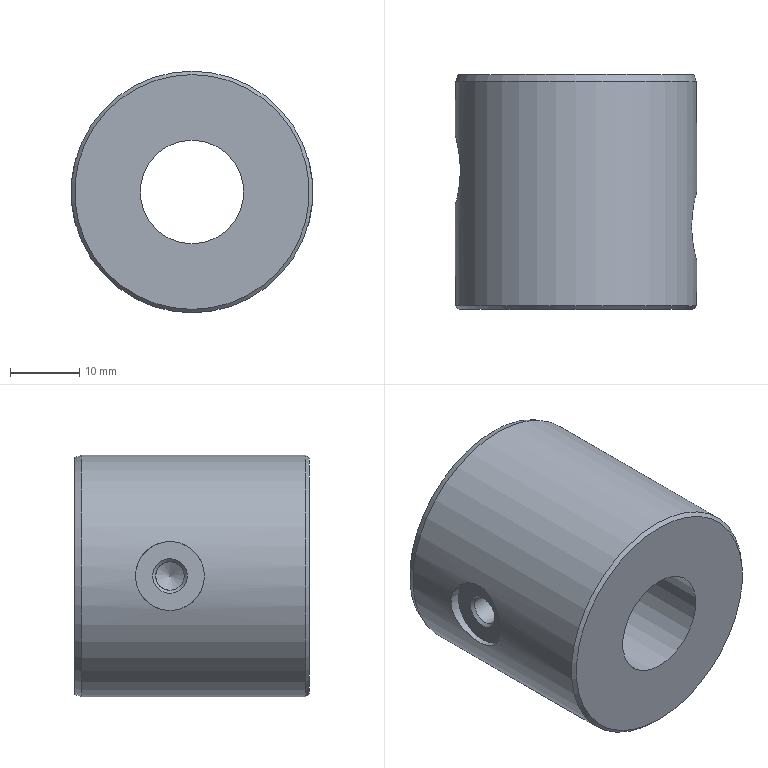Part | NX | 1 solid | 22 faces | box 35 x 34 x 35 mm | volume 26297 mm3 | cone 10 | cylinder 8 | plane 4 | commonest cylinder face diameters 2.459 x2 4.134 x2 10 x2 15 x1 35 x1
STEP:
#1=CARTESIAN_POINT('',(0.,14.5,-17.5));
#2=VERTEX_POINT('',#1);
#3=CARTESIAN_POINT('',(0.,14.5,0.));
#4=DIRECTION('',(0.,-1.,0.));
#5=DIRECTION('',(0.,0.,-1.));
#6=AXIS2_PLACEMENT_3D('',#3,#4,#5);
#7=CIRCLE('',#6,17.5);
#8=EDGE_CURVE('',#2,#2,#7,.F.);
#9=ORIENTED_EDGE('',*,*,#8,.T.);
#10=EDGE_LOOP('',(#9));
#11=FACE_BOUND('',#10,.T.);
#12=CARTESIAN_POINT('',(-17.5,29.2,0.));
#13=VERTEX_POINT('',#12);
#14=CARTESIAN_POINT('',(-17.142,30.283,3.921));
#15=CARTESIAN_POINT('',(-17.679,28.658,-0.000672));
#16=CARTESIAN_POINT('',(-17.143,30.285,-3.918));
#17=CARTESIAN_POINT('',(-16.584,34.192,-5.54));
#18=CARTESIAN_POINT('',(-17.142,38.117,-3.921));
#19=CARTESIAN_POINT('',(-17.679,39.742,-0.00000996));
#20=CARTESIAN_POINT('',(-17.143,38.116,3.918));
#21=CARTESIAN_POINT('',(-16.584,34.208,5.54));
#22=CARTESIAN_POINT('',(-17.142,30.283,3.921));
#23=CARTESIAN_POINT('',(-17.679,28.658,-0.000672));
#24=CARTESIAN_POINT('',(-17.143,30.285,-3.918));
#25=B_SPLINE_CURVE_WITH_KNOTS('',3,(#14,#15,#16,#17,#18,#19,#20,#21,#22,#23,#24),.UNSPECIFIED.,.T.,.F.,(1,1,1,1,1,1,1,1,1,1,1,1,1,1,1),(-0.01178,-0.007854,-0.003927,0.,0.003927,0.007854,0.01178,0.01571,0.01964,0.02356,0.02749,0.03142,0.03534,0.03927,0.0432),.UNSPECIFIED.);
#26=EDGE_CURVE('',#13,#13,#25,.T.);
#27=ORIENTED_EDGE('',*,*,#26,.T.);
#28=EDGE_LOOP('',(#27));
#29=FACE_BOUND('',#28,.T.);
#30=CARTESIAN_POINT('',(0.,47.,-17.5));
#31=VERTEX_POINT('',#30);
#32=CARTESIAN_POINT('',(0.,47.,0.));
#33=DIRECTION('',(0.,-1.,0.));
#34=DIRECTION('',(0.,0.,-1.));
#35=AXIS2_PLACEMENT_3D('',#32,#33,#34);
#36=CIRCLE('',#35,17.5);
#37=EDGE_CURVE('',#31,#31,#36,.T.);
#38=ORIENTED_EDGE('',*,*,#37,.T.);
#39=EDGE_LOOP('',(#38));
#40=FACE_BOUND('',#39,.T.);
#41=CARTESIAN_POINT('',(17.5,31.,0.));
#42=VERTEX_POINT('',#41);
#43=CARTESIAN_POINT('',(17.142,29.917,3.921));
#44=CARTESIAN_POINT('',(17.679,31.542,-0.000672));
#45=CARTESIAN_POINT('',(17.143,29.915,-3.918));
#46=CARTESIAN_POINT('',(16.584,26.008,-5.54));
#47=CARTESIAN_POINT('',(17.142,22.083,-3.921));
#48=CARTESIAN_POINT('',(17.679,20.458,-0.00000996));
#49=CARTESIAN_POINT('',(17.143,22.084,3.918));
#50=CARTESIAN_POINT('',(16.584,25.992,5.54));
#51=CARTESIAN_POINT('',(17.142,29.917,3.921));
#52=CARTESIAN_POINT('',(17.679,31.542,-0.000672));
#53=CARTESIAN_POINT('',(17.143,29.915,-3.918));
#54=B_SPLINE_CURVE_WITH_KNOTS('',3,(#43,#44,#45,#46,#47,#48,#49,#50,#51,#52,#53),.UNSPECIFIED.,.T.,.F.,(1,1,1,1,1,1,1,1,1,1,1,1,1,1,1),(-0.01178,-0.007854,-0.003927,0.,0.003927,0.007854,0.01178,0.01571,0.01964,0.02356,0.02749,0.03142,0.03534,0.03927,0.0432),.UNSPECIFIED.);
#55=EDGE_CURVE('',#42,#42,#54,.T.);
#56=ORIENTED_EDGE('',*,*,#55,.T.);
#57=EDGE_LOOP('',(#56));
#58=FACE_BOUND('',#57,.T.);
#59=CARTESIAN_POINT('',(0.,30.75,0.));
#60=DIRECTION('',(0.,-1.,0.));
#61=DIRECTION('',(0.,0.,-1.));
#62=AXIS2_PLACEMENT_3D('',#59,#60,#61);
#63=CYLINDRICAL_SURFACE('',#62,17.5);
#64=ADVANCED_FACE('',(#11,#29,#40,#58),#63,.T.);
#65=ORIENTED_EDGE('',*,*,#55,.F.);
#66=EDGE_LOOP('',(#65));
#67=FACE_BOUND('',#66,.T.);
#68=CARTESIAN_POINT('',(16.,26.,-5.));
#69=VERTEX_POINT('',#68);
#70=CARTESIAN_POINT('',(16.,26.,0.));
#71=DIRECTION('',(1.,0.,0.));
#72=DIRECTION('',(0.,0.,-1.));
#73=AXIS2_PLACEMENT_3D('',#70,#71,#72);
#74=CIRCLE('',#73,5.);
#75=EDGE_CURVE('',#69,#69,#74,.T.);
#76=ORIENTED_EDGE('',*,*,#75,.F.);
#77=EDGE_LOOP('',(#76));
#78=FACE_BOUND('',#77,.T.);
#79=CARTESIAN_POINT('',(16.75,26.,0.));
#80=DIRECTION('',(1.,0.,0.));
#81=DIRECTION('',(0.,0.,-1.));
#82=AXIS2_PLACEMENT_3D('',#79,#80,#81);
#83=CYLINDRICAL_SURFACE('',#82,5.);
#84=ADVANCED_FACE('',(#67,#78),#83,.F.);
#85=ORIENTED_EDGE('',*,*,#37,.F.);
#86=EDGE_LOOP('',(#85));
#87=FACE_BOUND('',#86,.T.);
#88=CARTESIAN_POINT('',(0.,48.,-17.14));
#89=VERTEX_POINT('',#88);
#90=CARTESIAN_POINT('',(0.,48.,0.));
#91=DIRECTION('',(0.,-1.,0.));
#92=DIRECTION('',(0.,0.,-1.));
#93=AXIS2_PLACEMENT_3D('',#90,#91,#92);
#94=CIRCLE('',#93,17.14);
#95=EDGE_CURVE('',#89,#89,#94,.T.);
#96=ORIENTED_EDGE('',*,*,#95,.T.);
#97=EDGE_LOOP('',(#96));
#98=FACE_BOUND('',#97,.T.);
#99=CARTESIAN_POINT('',(0.,47.,0.));
#100=DIRECTION('',(0.,-1.,0.));
#101=DIRECTION('',(0.,0.,-1.));
#102=AXIS2_PLACEMENT_3D('',#99,#100,#101);
#103=CONICAL_SURFACE('',#102,17.5,0.3456);
#104=ADVANCED_FACE('',(#87,#98),#103,.T.);
#105=ORIENTED_EDGE('',*,*,#26,.F.);
#106=EDGE_LOOP('',(#105));
#107=FACE_BOUND('',#106,.T.);
#108=CARTESIAN_POINT('',(-16.,34.2,-5.));
#109=VERTEX_POINT('',#108);
#110=CARTESIAN_POINT('',(-16.,34.2,0.));
#111=DIRECTION('',(1.,0.,0.));
#112=DIRECTION('',(0.,0.,-1.));
#113=AXIS2_PLACEMENT_3D('',#110,#111,#112);
#114=CIRCLE('',#113,5.);
#115=EDGE_CURVE('',#109,#109,#114,.F.);
#116=ORIENTED_EDGE('',*,*,#115,.F.);
#117=EDGE_LOOP('',(#116));
#118=FACE_BOUND('',#117,.T.);
#119=CARTESIAN_POINT('',(-16.75,34.2,0.));
#120=DIRECTION('',(1.,0.,0.));
#121=DIRECTION('',(0.,0.,-1.));
#122=AXIS2_PLACEMENT_3D('',#119,#120,#121);
#123=CYLINDRICAL_SURFACE('',#122,5.);
#124=ADVANCED_FACE('',(#107,#118),#123,.F.);
#125=CARTESIAN_POINT('',(0.,14.,17.));
#126=VERTEX_POINT('',#125);
#127=CARTESIAN_POINT('',(0.,14.,0.));
#128=DIRECTION('',(0.,1.,0.));
#129=DIRECTION('',(0.,0.,1.));
#130=AXIS2_PLACEMENT_3D('',#127,#128,#129);
#131=CIRCLE('',#130,17.);
#132=EDGE_CURVE('',#126,#126,#131,.T.);
#133=ORIENTED_EDGE('',*,*,#132,.T.);
#134=EDGE_LOOP('',(#133));
#135=FACE_BOUND('',#134,.T.);
#136=ORIENTED_EDGE('',*,*,#8,.F.);
#137=EDGE_LOOP('',(#136));
#138=FACE_BOUND('',#137,.T.);
#139=CARTESIAN_POINT('',(0.,14.5,0.));
#140=DIRECTION('',(0.,1.,0.));
#141=DIRECTION('',(0.,0.,1.));
#142=AXIS2_PLACEMENT_3D('',#139,#140,#141);
#143=CONICAL_SURFACE('',#142,17.5,0.7854);
#144=ADVANCED_FACE('',(#135,#138),#143,.T.);
#145=ORIENTED_EDGE('',*,*,#75,.T.);
#146=EDGE_LOOP('',(#145));
#147=FACE_BOUND('',#146,.T.);
#148=CARTESIAN_POINT('',(16.,26.,-2.5));
#149=VERTEX_POINT('',#148);
#150=CARTESIAN_POINT('',(16.,26.,0.));
#151=DIRECTION('',(1.,0.,0.));
#152=DIRECTION('',(0.,0.,-1.));
#153=AXIS2_PLACEMENT_3D('',#150,#151,#152);
#154=CIRCLE('',#153,2.5);
#155=EDGE_CURVE('',#149,#149,#154,.T.);
#156=ORIENTED_EDGE('',*,*,#155,.F.);
#157=EDGE_LOOP('',(#156));
#158=FACE_BOUND('',#157,.T.);
#159=CARTESIAN_POINT('',(16.,29.75,0.));
#160=DIRECTION('',(-1.,0.,0.));
#161=DIRECTION('',(0.,0.,1.));
#162=AXIS2_PLACEMENT_3D('',#159,#160,#161);
#163=PLANE('',#162);
#164=ADVANCED_FACE('',(#147,#158),#163,.F.);
#165=ORIENTED_EDGE('',*,*,#95,.F.);
#166=EDGE_LOOP('',(#165));
#167=FACE_BOUND('',#166,.T.);
#168=CARTESIAN_POINT('',(0.,48.,-7.5));
#169=VERTEX_POINT('',#168);
#170=CARTESIAN_POINT('',(0.,48.,0.));
#171=DIRECTION('',(0.,-1.,0.));
#172=DIRECTION('',(0.,0.,-1.));
#173=AXIS2_PLACEMENT_3D('',#170,#171,#172);
#174=CIRCLE('',#173,7.5);
#175=EDGE_CURVE('',#169,#169,#174,.T.);
#176=ORIENTED_EDGE('',*,*,#175,.T.);
#177=EDGE_LOOP('',(#176));
#178=FACE_BOUND('',#177,.T.);
#179=CARTESIAN_POINT('',(0.,48.,16.));
#180=VERTEX_POINT('',#179);
#181=CARTESIAN_POINT('',(0.,48.,14.5));
#182=DIRECTION('',(0.,1.,0.));
#183=DIRECTION('',(0.,0.,1.));
#184=AXIS2_PLACEMENT_3D('',#181,#182,#183);
#185=CIRCLE('',#184,1.5);
#186=EDGE_CURVE('',#180,#180,#185,.F.);
#187=ORIENTED_EDGE('',*,*,#186,.T.);
#188=EDGE_LOOP('',(#187));
#189=FACE_BOUND('',#188,.T.);
#190=CARTESIAN_POINT('',(0.,48.,-13.));
#191=VERTEX_POINT('',#190);
#192=CARTESIAN_POINT('',(0.,48.,-14.5));
#193=DIRECTION('',(0.,1.,0.));
#194=DIRECTION('',(0.,0.,1.));
#195=AXIS2_PLACEMENT_3D('',#192,#193,#194);
#196=CIRCLE('',#195,1.5);
#197=EDGE_CURVE('',#191,#191,#196,.F.);
#198=ORIENTED_EDGE('',*,*,#197,.T.);
#199=EDGE_LOOP('',(#198));
#200=FACE_BOUND('',#199,.T.);
#201=CARTESIAN_POINT('',(12.32,48.,0.));
#202=DIRECTION('',(0.,1.,0.));
#203=DIRECTION('',(0.,0.,1.));
#204=AXIS2_PLACEMENT_3D('',#201,#202,#203);
#205=PLANE('',#204);
#206=ADVANCED_FACE('',(#167,#178,#189,#200),#205,.T.);
#207=CARTESIAN_POINT('',(-16.,34.2,2.5));
#208=VERTEX_POINT('',#207);
#209=CARTESIAN_POINT('',(-16.,34.2,0.));
#210=DIRECTION('',(-1.,0.,0.));
#211=DIRECTION('',(0.,0.,1.));
#212=AXIS2_PLACEMENT_3D('',#209,#210,#211);
#213=CIRCLE('',#212,2.5);
#214=EDGE_CURVE('',#208,#208,#213,.T.);
#215=ORIENTED_EDGE('',*,*,#214,.F.);
#216=EDGE_LOOP('',(#215));
#217=FACE_BOUND('',#216,.T.);
#218=ORIENTED_EDGE('',*,*,#115,.T.);
#219=EDGE_LOOP('',(#218));
#220=FACE_BOUND('',#219,.T.);
#221=CARTESIAN_POINT('',(-16.,37.95,0.));
#222=DIRECTION('',(1.,0.,0.));
#223=DIRECTION('',(0.,0.,-1.));
#224=AXIS2_PLACEMENT_3D('',#221,#222,#223);
#225=PLANE('',#224);
#226=ADVANCED_FACE('',(#217,#220),#225,.F.);
#227=CARTESIAN_POINT('',(0.,14.,-7.5));
#228=VERTEX_POINT('',#227);
#229=CARTESIAN_POINT('',(0.,14.,0.));
#230=DIRECTION('',(0.,-1.,0.));
#231=DIRECTION('',(0.,0.,-1.));
#232=AXIS2_PLACEMENT_3D('',#229,#230,#231);
#233=CIRCLE('',#232,7.5);
#234=EDGE_CURVE('',#228,#228,#233,.F.);
#235=ORIENTED_EDGE('',*,*,#234,.T.);
#236=EDGE_LOOP('',(#235));
#237=FACE_BOUND('',#236,.T.);
#238=ORIENTED_EDGE('',*,*,#132,.F.);
#239=EDGE_LOOP('',(#238));
#240=FACE_BOUND('',#239,.T.);
#241=CARTESIAN_POINT('',(12.25,14.,0.));
#242=DIRECTION('',(0.,-1.,0.));
#243=DIRECTION('',(0.,0.,-1.));
#244=AXIS2_PLACEMENT_3D('',#241,#242,#243);
#245=PLANE('',#244);
#246=ADVANCED_FACE('',(#237,#240),#245,.T.);
#247=CARTESIAN_POINT('',(15.567,28.067,0.));
#248=VERTEX_POINT('',#247);
#249=CARTESIAN_POINT('',(15.567,26.,0.));
#250=DIRECTION('',(1.,0.,0.));
#251=DIRECTION('',(0.,1.,0.));
#252=AXIS2_PLACEMENT_3D('',#249,#250,#251);
#253=CIRCLE('',#252,2.067);
#254=EDGE_CURVE('',#248,#248,#253,.T.);
#255=ORIENTED_EDGE('',*,*,#254,.F.);
#256=EDGE_LOOP('',(#255));
#257=FACE_BOUND('',#256,.T.);
#258=ORIENTED_EDGE('',*,*,#155,.T.);
#259=EDGE_LOOP('',(#258));
#260=FACE_BOUND('',#259,.T.);
#261=CARTESIAN_POINT('',(16.,26.,0.));
#262=DIRECTION('',(1.,0.,0.));
#263=DIRECTION('',(0.,0.,-1.));
#264=AXIS2_PLACEMENT_3D('',#261,#262,#263);
#265=CONICAL_SURFACE('',#264,2.5,0.7854);
#266=ADVANCED_FACE('',(#257,#260),#265,.F.);
#267=ORIENTED_EDGE('',*,*,#234,.F.);
#268=EDGE_LOOP('',(#267));
#269=FACE_BOUND('',#268,.T.);
#270=ORIENTED_EDGE('',*,*,#175,.F.);
#271=EDGE_LOOP('',(#270));
#272=FACE_BOUND('',#271,.T.);
#273=CARTESIAN_POINT('',(0.,31.,0.));
#274=DIRECTION('',(0.,-1.,0.));
#275=DIRECTION('',(0.,0.,-1.));
#276=AXIS2_PLACEMENT_3D('',#273,#274,#275);
#277=CYLINDRICAL_SURFACE('',#276,7.5);
#278=ADVANCED_FACE('',(#269,#272),#277,.F.);
#279=ORIENTED_EDGE('',*,*,#186,.F.);
#280=EDGE_LOOP('',(#279));
#281=FACE_BOUND('',#280,.T.);
#282=CARTESIAN_POINT('',(0.,47.73,15.73));
#283=VERTEX_POINT('',#282);
#284=CARTESIAN_POINT('',(0.,47.73,14.5));
#285=DIRECTION('',(0.,1.,0.));
#286=DIRECTION('',(0.,0.,1.));
#287=AXIS2_PLACEMENT_3D('',#284,#285,#286);
#288=CIRCLE('',#287,1.23);
#289=EDGE_CURVE('',#283,#283,#288,.T.);
#290=ORIENTED_EDGE('',*,*,#289,.F.);
#291=EDGE_LOOP('',(#290));
#292=FACE_BOUND('',#291,.T.);
#293=CARTESIAN_POINT('',(0.,48.,14.5));
#294=DIRECTION('',(0.,1.,0.));
#295=DIRECTION('',(0.,0.,1.));
#296=AXIS2_PLACEMENT_3D('',#293,#294,#295);
#297=CONICAL_SURFACE('',#296,1.5,0.7854);
#298=ADVANCED_FACE('',(#281,#292),#297,.F.);
#299=ORIENTED_EDGE('',*,*,#197,.F.);
#300=EDGE_LOOP('',(#299));
#301=FACE_BOUND('',#300,.T.);
#302=CARTESIAN_POINT('',(0.,47.73,-13.27));
#303=VERTEX_POINT('',#302);
#304=CARTESIAN_POINT('',(0.,47.73,-14.5));
#305=DIRECTION('',(0.,1.,0.));
#306=DIRECTION('',(0.,0.,1.));
#307=AXIS2_PLACEMENT_3D('',#304,#305,#306);
#308=CIRCLE('',#307,1.23);
#309=EDGE_CURVE('',#303,#303,#308,.T.);
#310=ORIENTED_EDGE('',*,*,#309,.F.);
#311=EDGE_LOOP('',(#310));
#312=FACE_BOUND('',#311,.T.);
#313=CARTESIAN_POINT('',(0.,48.,-14.5));
#314=DIRECTION('',(0.,1.,0.));
#315=DIRECTION('',(0.,0.,1.));
#316=AXIS2_PLACEMENT_3D('',#313,#314,#315);
#317=CONICAL_SURFACE('',#316,1.5,0.7854);
#318=ADVANCED_FACE('',(#301,#312),#317,.F.);
#319=ORIENTED_EDGE('',*,*,#214,.T.);
#320=EDGE_LOOP('',(#319));
#321=FACE_BOUND('',#320,.T.);
#322=CARTESIAN_POINT('',(-15.567,36.267,0.));
#323=VERTEX_POINT('',#322);
#324=CARTESIAN_POINT('',(-15.567,34.2,0.));
#325=DIRECTION('',(-1.,0.,0.));
#326=DIRECTION('',(0.,1.,0.));
#327=AXIS2_PLACEMENT_3D('',#324,#325,#326);
#328=CIRCLE('',#327,2.067);
#329=EDGE_CURVE('',#323,#323,#328,.T.);
#330=ORIENTED_EDGE('',*,*,#329,.F.);
#331=EDGE_LOOP('',(#330));
#332=FACE_BOUND('',#331,.T.);
#333=CARTESIAN_POINT('',(-16.,34.2,0.));
#334=DIRECTION('',(-1.,0.,0.));
#335=DIRECTION('',(0.,0.,1.));
#336=AXIS2_PLACEMENT_3D('',#333,#334,#335);
#337=CONICAL_SURFACE('',#336,2.5,0.7854);
#338=ADVANCED_FACE('',(#321,#332),#337,.F.);
#339=CARTESIAN_POINT('',(12.5,26.,-2.067));
#340=VERTEX_POINT('',#339);
#341=CARTESIAN_POINT('',(12.5,26.,0.));
#342=DIRECTION('',(1.,0.,0.));
#343=DIRECTION('',(0.,0.,-1.));
#344=AXIS2_PLACEMENT_3D('',#341,#342,#343);
#345=CIRCLE('',#344,2.067);
#346=EDGE_CURVE('',#340,#340,#345,.T.);
#347=ORIENTED_EDGE('',*,*,#346,.F.);
#348=EDGE_LOOP('',(#347));
#349=FACE_BOUND('',#348,.T.);
#350=ORIENTED_EDGE('',*,*,#254,.T.);
#351=EDGE_LOOP('',(#350));
#352=FACE_BOUND('',#351,.T.);
#353=CARTESIAN_POINT('',(14.034,26.,0.));
#354=DIRECTION('',(1.,0.,0.));
#355=DIRECTION('',(0.,0.,-1.));
#356=AXIS2_PLACEMENT_3D('',#353,#354,#355);
#357=CYLINDRICAL_SURFACE('',#356,2.067);
#358=ADVANCED_FACE('',(#349,#352),#357,.F.);
#359=ORIENTED_EDGE('',*,*,#289,.T.);
#360=EDGE_LOOP('',(#359));
#361=FACE_BOUND('',#360,.T.);
#362=CARTESIAN_POINT('',(0.,42.,15.729));
#363=VERTEX_POINT('',#362);
#364=CARTESIAN_POINT('',(0.,42.,14.5));
#365=DIRECTION('',(0.,1.,0.));
#366=DIRECTION('',(0.,0.,1.));
#367=AXIS2_PLACEMENT_3D('',#364,#365,#366);
#368=CIRCLE('',#367,1.23);
#369=EDGE_CURVE('',#363,#363,#368,.T.);
#370=ORIENTED_EDGE('',*,*,#369,.F.);
#371=EDGE_LOOP('',(#370));
#372=FACE_BOUND('',#371,.T.);
#373=CARTESIAN_POINT('',(0.,44.865,14.5));
#374=DIRECTION('',(0.,1.,0.));
#375=DIRECTION('',(0.,0.,1.));
#376=AXIS2_PLACEMENT_3D('',#373,#374,#375);
#377=CYLINDRICAL_SURFACE('',#376,1.23);
#378=ADVANCED_FACE('',(#361,#372),#377,.F.);
#379=ORIENTED_EDGE('',*,*,#309,.T.);
#380=EDGE_LOOP('',(#379));
#381=FACE_BOUND('',#380,.T.);
#382=CARTESIAN_POINT('',(0.,42.,-13.271));
#383=VERTEX_POINT('',#382);
#384=CARTESIAN_POINT('',(0.,42.,-14.5));
#385=DIRECTION('',(0.,1.,0.));
#386=DIRECTION('',(0.,0.,1.));
#387=AXIS2_PLACEMENT_3D('',#384,#385,#386);
#388=CIRCLE('',#387,1.23);
#389=EDGE_CURVE('',#383,#383,#388,.T.);
#390=ORIENTED_EDGE('',*,*,#389,.F.);
#391=EDGE_LOOP('',(#390));
#392=FACE_BOUND('',#391,.T.);
#393=CARTESIAN_POINT('',(0.,44.865,-14.5));
#394=DIRECTION('',(0.,1.,0.));
#395=DIRECTION('',(0.,0.,1.));
#396=AXIS2_PLACEMENT_3D('',#393,#394,#395);
#397=CYLINDRICAL_SURFACE('',#396,1.23);
#398=ADVANCED_FACE('',(#381,#392),#397,.F.);
#399=ORIENTED_EDGE('',*,*,#329,.T.);
#400=EDGE_LOOP('',(#399));
#401=FACE_BOUND('',#400,.T.);
#402=CARTESIAN_POINT('',(-12.5,34.2,-2.067));
#403=VERTEX_POINT('',#402);
#404=CARTESIAN_POINT('',(-12.5,34.2,0.));
#405=DIRECTION('',(1.,0.,0.));
#406=DIRECTION('',(0.,0.,-1.));
#407=AXIS2_PLACEMENT_3D('',#404,#405,#406);
#408=CIRCLE('',#407,2.067);
#409=EDGE_CURVE('',#403,#403,#408,.F.);
#410=ORIENTED_EDGE('',*,*,#409,.F.);
#411=EDGE_LOOP('',(#410));
#412=FACE_BOUND('',#411,.T.);
#413=CARTESIAN_POINT('',(-14.034,34.2,0.));
#414=DIRECTION('',(1.,0.,0.));
#415=DIRECTION('',(0.,0.,-1.));
#416=AXIS2_PLACEMENT_3D('',#413,#414,#415);
#417=CYLINDRICAL_SURFACE('',#416,2.067);
#418=ADVANCED_FACE('',(#401,#412),#417,.F.);
#419=ORIENTED_EDGE('',*,*,#346,.T.);
#420=EDGE_LOOP('',(#419));
#421=FACE_BOUND('',#420,.T.);
#422=CARTESIAN_POINT('',(11.307,26.,0.));
#423=VERTEX_POINT('',#422);
#424=VERTEX_LOOP('',#423);
#425=FACE_BOUND('',#424,.T.);
#426=CARTESIAN_POINT('',(12.5,26.,0.));
#427=DIRECTION('',(1.,0.,0.));
#428=DIRECTION('',(0.,0.,-1.));
#429=AXIS2_PLACEMENT_3D('',#426,#427,#428);
#430=CONICAL_SURFACE('',#429,2.067,1.047);
#431=ADVANCED_FACE('',(#421,#425),#430,.F.);
#432=CARTESIAN_POINT('',(0.,41.29,14.5));
#433=VERTEX_POINT('',#432);
#434=VERTEX_LOOP('',#433);
#435=FACE_BOUND('',#434,.T.);
#436=ORIENTED_EDGE('',*,*,#369,.T.);
#437=EDGE_LOOP('',(#436));
#438=FACE_BOUND('',#437,.T.);
#439=CARTESIAN_POINT('',(0.,42.,14.5));
#440=DIRECTION('',(0.,1.,0.));
#441=DIRECTION('',(0.,0.,1.));
#442=AXIS2_PLACEMENT_3D('',#439,#440,#441);
#443=CONICAL_SURFACE('',#442,1.23,1.047);
#444=ADVANCED_FACE('',(#435,#438),#443,.F.);
#445=CARTESIAN_POINT('',(0.,41.29,-14.5));
#446=VERTEX_POINT('',#445);
#447=VERTEX_LOOP('',#446);
#448=FACE_BOUND('',#447,.T.);
#449=ORIENTED_EDGE('',*,*,#389,.T.);
#450=EDGE_LOOP('',(#449));
#451=FACE_BOUND('',#450,.T.);
#452=CARTESIAN_POINT('',(0.,42.,-14.5));
#453=DIRECTION('',(0.,1.,0.));
#454=DIRECTION('',(0.,0.,1.));
#455=AXIS2_PLACEMENT_3D('',#452,#453,#454);
#456=CONICAL_SURFACE('',#455,1.229,1.047);
#457=ADVANCED_FACE('',(#448,#451),#456,.F.);
#458=CARTESIAN_POINT('',(-11.307,34.2,0.));
#459=VERTEX_POINT('',#458);
#460=VERTEX_LOOP('',#459);
#461=FACE_BOUND('',#460,.T.);
#462=ORIENTED_EDGE('',*,*,#409,.T.);
#463=EDGE_LOOP('',(#462));
#464=FACE_BOUND('',#463,.T.);
#465=CARTESIAN_POINT('',(-12.5,34.2,0.));
#466=DIRECTION('',(-1.,0.,0.));
#467=DIRECTION('',(0.,0.,1.));
#468=AXIS2_PLACEMENT_3D('',#465,#466,#467);
#469=CONICAL_SURFACE('',#468,2.067,1.047);
#470=ADVANCED_FACE('',(#461,#464),#469,.F.);
#471=CLOSED_SHELL('',(#64,#84,#104,#124,#144,#164,#206,#226,#246,#266,#278,#298,#318,#338,#358,#378,#398,#418,#431,#444,#457,#470));
#472=MANIFOLD_SOLID_BREP('',#471);
#473=(LENGTH_UNIT()NAMED_UNIT(*)SI_UNIT(.MILLI.,.METRE.));
#474=UNCERTAINTY_MEASURE_WITH_UNIT(LENGTH_MEASURE(0.0508),#473,'','');
#475=(NAMED_UNIT(*)PLANE_ANGLE_UNIT()SI_UNIT($,.RADIAN.));
#476=(NAMED_UNIT(*)SI_UNIT($,.STERADIAN.)SOLID_ANGLE_UNIT());
#477=(GEOMETRIC_REPRESENTATION_CONTEXT(3)GLOBAL_UNCERTAINTY_ASSIGNED_CONTEXT((#474))GLOBAL_UNIT_ASSIGNED_CONTEXT((#473,#475,#476))REPRESENTATION_CONTEXT('',''));
#478=ADVANCED_BREP_SHAPE_REPRESENTATION('',(#472),#477);